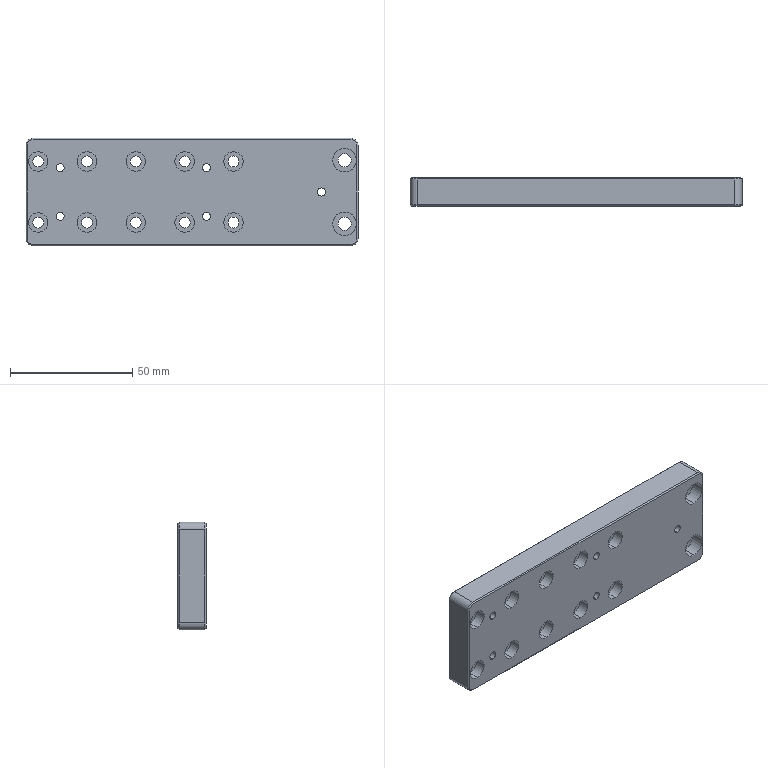Part | STEP file | Guide wheel mechanism revised.sldasm-Part-45 | 1 solid | 96 faces | box 136 x 11.6 x 44 mm | volume 64318 mm3 | cylinder 62 | plane 26 | cone 8 | commonest cylinder face diameters 4.5 x20 8 x20 3.3 x10 5.4 x4 6 x4 9.6 x4